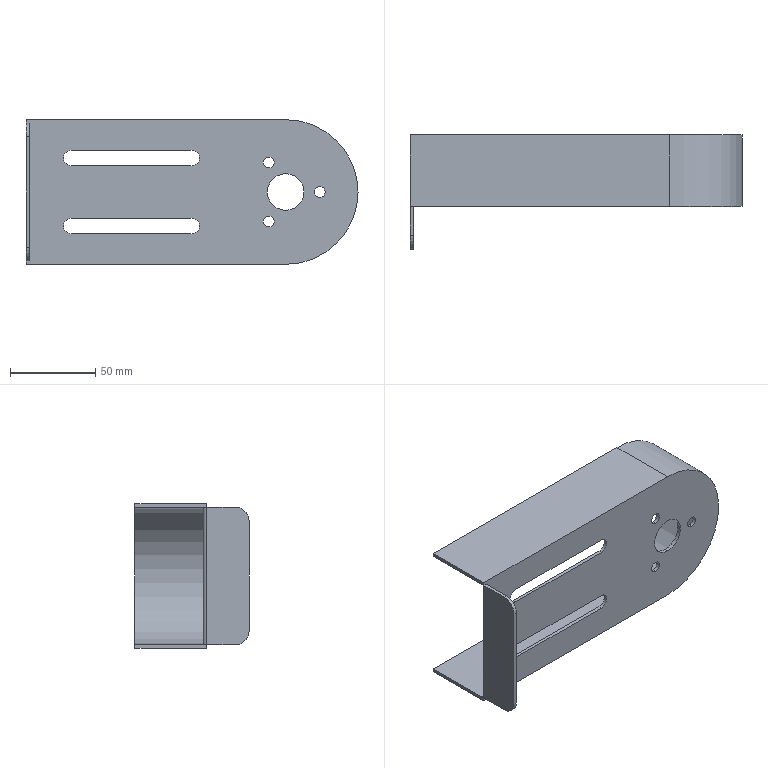Part | STEP file | 1.6米轴盖 | 1 solid | 35 faces | box 195 x 67 x 85 mm | volume 66626 mm3 | plane 18 | cylinder 17 | commonest cylinder face diameters 6.4 x6 9 x4 16 x2 21.5 x2 4 x1 81 x1
STEP:
#1=CARTESIAN_POINT('',(142.5,2.,-21.979));
#2=VERTEX_POINT('',#1);
#3=CARTESIAN_POINT('',(142.5,2.,-28.379));
#4=VERTEX_POINT('',#3);
#5=CARTESIAN_POINT('',(142.5,2.,-25.179));
#6=DIRECTION('',(0.,-1.,0.));
#7=DIRECTION('',(0.,0.,-1.));
#8=AXIS2_PLACEMENT_3D('',#5,#6,#7);
#9=CIRCLE('',#8,3.2);
#10=EDGE_CURVE('',#2,#4,#9,.T.);
#11=ORIENTED_EDGE('',*,*,#10,.F.);
#12=CARTESIAN_POINT('',(142.5,0.,-21.979));
#13=VERTEX_POINT('',#12);
#14=CARTESIAN_POINT('',(142.5,2.,-21.979));
#15=DIRECTION('',(0.,-1.,0.));
#16=VECTOR('',#15,1000.);
#17=LINE('',#14,#16);
#18=EDGE_CURVE('',#2,#13,#17,.T.);
#19=ORIENTED_EDGE('',*,*,#18,.T.);
#20=CARTESIAN_POINT('',(142.5,0.,-28.379));
#21=VERTEX_POINT('',#20);
#22=CARTESIAN_POINT('',(142.5,0.,-25.179));
#23=DIRECTION('',(0.,-1.,0.));
#24=DIRECTION('',(0.,0.,-1.));
#25=AXIS2_PLACEMENT_3D('',#22,#23,#24);
#26=CIRCLE('',#25,3.2);
#27=EDGE_CURVE('',#13,#21,#26,.T.);
#28=ORIENTED_EDGE('',*,*,#27,.T.);
#29=CARTESIAN_POINT('',(142.5,2.,-28.379));
#30=DIRECTION('',(0.,-1.,0.));
#31=VECTOR('',#30,1000.);
#32=LINE('',#29,#31);
#33=EDGE_CURVE('',#4,#21,#32,.T.);
#34=ORIENTED_EDGE('',*,*,#33,.F.);
#35=EDGE_LOOP('',(#11,#19,#28,#34));
#36=FACE_OUTER_BOUND('',#35,.T.);
#37=CARTESIAN_POINT('',(142.5,2.,-25.179));
#38=DIRECTION('',(0.,-1.,0.));
#39=DIRECTION('',(0.,0.,-1.));
#40=AXIS2_PLACEMENT_3D('',#37,#38,#39);
#41=CYLINDRICAL_SURFACE('',#40,3.2);
#42=ADVANCED_FACE('',(#36),#41,.F.);
#43=CARTESIAN_POINT('',(142.5,2.,-56.621));
#44=VERTEX_POINT('',#43);
#45=CARTESIAN_POINT('',(142.5,2.,-63.021));
#46=VERTEX_POINT('',#45);
#47=CARTESIAN_POINT('',(142.5,2.,-59.821));
#48=DIRECTION('',(0.,-1.,0.));
#49=DIRECTION('',(0.,0.,-1.));
#50=AXIS2_PLACEMENT_3D('',#47,#48,#49);
#51=CIRCLE('',#50,3.2);
#52=EDGE_CURVE('',#44,#46,#51,.T.);
#53=ORIENTED_EDGE('',*,*,#52,.F.);
#54=CARTESIAN_POINT('',(142.5,0.,-56.621));
#55=VERTEX_POINT('',#54);
#56=CARTESIAN_POINT('',(142.5,2.,-56.621));
#57=DIRECTION('',(0.,-1.,0.));
#58=VECTOR('',#57,1000.);
#59=LINE('',#56,#58);
#60=EDGE_CURVE('',#44,#55,#59,.T.);
#61=ORIENTED_EDGE('',*,*,#60,.T.);
#62=CARTESIAN_POINT('',(142.5,0.,-63.021));
#63=VERTEX_POINT('',#62);
#64=CARTESIAN_POINT('',(142.5,0.,-59.821));
#65=DIRECTION('',(0.,-1.,0.));
#66=DIRECTION('',(0.,0.,-1.));
#67=AXIS2_PLACEMENT_3D('',#64,#65,#66);
#68=CIRCLE('',#67,3.2);
#69=EDGE_CURVE('',#55,#63,#68,.T.);
#70=ORIENTED_EDGE('',*,*,#69,.T.);
#71=CARTESIAN_POINT('',(142.5,2.,-63.021));
#72=DIRECTION('',(0.,-1.,0.));
#73=VECTOR('',#72,1000.);
#74=LINE('',#71,#73);
#75=EDGE_CURVE('',#46,#63,#74,.T.);
#76=ORIENTED_EDGE('',*,*,#75,.F.);
#77=EDGE_LOOP('',(#53,#61,#70,#76));
#78=FACE_OUTER_BOUND('',#77,.T.);
#79=CARTESIAN_POINT('',(142.5,2.,-59.821));
#80=DIRECTION('',(0.,-1.,0.));
#81=DIRECTION('',(0.,0.,-1.));
#82=AXIS2_PLACEMENT_3D('',#79,#80,#81);
#83=CYLINDRICAL_SURFACE('',#82,3.2);
#84=ADVANCED_FACE('',(#78),#83,.F.);
#85=CARTESIAN_POINT('',(172.5,2.,-39.3));
#86=VERTEX_POINT('',#85);
#87=CARTESIAN_POINT('',(172.5,2.,-45.7));
#88=VERTEX_POINT('',#87);
#89=CARTESIAN_POINT('',(172.5,2.,-42.5));
#90=DIRECTION('',(0.,-1.,0.));
#91=DIRECTION('',(0.,0.,-1.));
#92=AXIS2_PLACEMENT_3D('',#89,#90,#91);
#93=CIRCLE('',#92,3.2);
#94=EDGE_CURVE('',#86,#88,#93,.T.);
#95=ORIENTED_EDGE('',*,*,#94,.F.);
#96=CARTESIAN_POINT('',(172.5,0.,-39.3));
#97=VERTEX_POINT('',#96);
#98=CARTESIAN_POINT('',(172.5,2.,-39.3));
#99=DIRECTION('',(0.,-1.,0.));
#100=VECTOR('',#99,1000.);
#101=LINE('',#98,#100);
#102=EDGE_CURVE('',#86,#97,#101,.T.);
#103=ORIENTED_EDGE('',*,*,#102,.T.);
#104=CARTESIAN_POINT('',(172.5,0.,-45.7));
#105=VERTEX_POINT('',#104);
#106=CARTESIAN_POINT('',(172.5,0.,-42.5));
#107=DIRECTION('',(0.,-1.,0.));
#108=DIRECTION('',(0.,0.,-1.));
#109=AXIS2_PLACEMENT_3D('',#106,#107,#108);
#110=CIRCLE('',#109,3.2);
#111=EDGE_CURVE('',#97,#105,#110,.T.);
#112=ORIENTED_EDGE('',*,*,#111,.T.);
#113=CARTESIAN_POINT('',(172.5,2.,-45.7));
#114=DIRECTION('',(0.,-1.,0.));
#115=VECTOR('',#114,1000.);
#116=LINE('',#113,#115);
#117=EDGE_CURVE('',#88,#105,#116,.T.);
#118=ORIENTED_EDGE('',*,*,#117,.F.);
#119=EDGE_LOOP('',(#95,#103,#112,#118));
#120=FACE_OUTER_BOUND('',#119,.T.);
#121=CARTESIAN_POINT('',(172.5,2.,-42.5));
#122=DIRECTION('',(0.,-1.,0.));
#123=DIRECTION('',(0.,0.,-1.));
#124=AXIS2_PLACEMENT_3D('',#121,#122,#123);
#125=CYLINDRICAL_SURFACE('',#124,3.2);
#126=ADVANCED_FACE('',(#120),#125,.F.);
#127=CARTESIAN_POINT('',(152.5,2.,-31.75));
#128=VERTEX_POINT('',#127);
#129=CARTESIAN_POINT('',(152.5,2.,-53.25));
#130=VERTEX_POINT('',#129);
#131=CARTESIAN_POINT('',(152.5,2.,-42.5));
#132=DIRECTION('',(0.,-1.,0.));
#133=DIRECTION('',(0.,0.,-1.));
#134=AXIS2_PLACEMENT_3D('',#131,#132,#133);
#135=CIRCLE('',#134,10.75);
#136=EDGE_CURVE('',#128,#130,#135,.T.);
#137=ORIENTED_EDGE('',*,*,#136,.F.);
#138=CARTESIAN_POINT('',(152.5,0.,-31.75));
#139=VERTEX_POINT('',#138);
#140=CARTESIAN_POINT('',(152.5,2.,-31.75));
#141=DIRECTION('',(0.,-1.,0.));
#142=VECTOR('',#141,1000.);
#143=LINE('',#140,#142);
#144=EDGE_CURVE('',#128,#139,#143,.T.);
#145=ORIENTED_EDGE('',*,*,#144,.T.);
#146=CARTESIAN_POINT('',(152.5,0.,-53.25));
#147=VERTEX_POINT('',#146);
#148=CARTESIAN_POINT('',(152.5,0.,-42.5));
#149=DIRECTION('',(0.,-1.,0.));
#150=DIRECTION('',(0.,0.,-1.));
#151=AXIS2_PLACEMENT_3D('',#148,#149,#150);
#152=CIRCLE('',#151,10.75);
#153=EDGE_CURVE('',#139,#147,#152,.T.);
#154=ORIENTED_EDGE('',*,*,#153,.T.);
#155=CARTESIAN_POINT('',(152.5,2.,-53.25));
#156=DIRECTION('',(0.,-1.,0.));
#157=VECTOR('',#156,1000.);
#158=LINE('',#155,#157);
#159=EDGE_CURVE('',#130,#147,#158,.T.);
#160=ORIENTED_EDGE('',*,*,#159,.F.);
#161=EDGE_LOOP('',(#137,#145,#154,#160));
#162=FACE_OUTER_BOUND('',#161,.T.);
#163=CARTESIAN_POINT('',(152.5,2.,-42.5));
#164=DIRECTION('',(0.,-1.,0.));
#165=DIRECTION('',(0.,0.,-1.));
#166=AXIS2_PLACEMENT_3D('',#163,#164,#165);
#167=CYLINDRICAL_SURFACE('',#166,10.75);
#168=ADVANCED_FACE('',(#162),#167,.F.);
#169=CARTESIAN_POINT('',(0.,0.,-2.));
#170=VERTEX_POINT('',#169);
#171=CARTESIAN_POINT('',(0.,42.,-2.));
#172=VERTEX_POINT('',#171);
#173=CARTESIAN_POINT('',(0.,2.,-2.));
#174=DIRECTION('',(0.,1.,0.));
#175=VECTOR('',#174,1000.);
#176=LINE('',#173,#175);
#177=EDGE_CURVE('',#170,#172,#176,.T.);
#178=ORIENTED_EDGE('',*,*,#177,.F.);
#179=CARTESIAN_POINT('',(0.,0.,0.));
#180=VERTEX_POINT('',#179);
#181=CARTESIAN_POINT('',(0.,0.,0.));
#182=DIRECTION('',(0.,0.,1.));
#183=VECTOR('',#182,1000.);
#184=LINE('',#181,#183);
#185=EDGE_CURVE('',#170,#180,#184,.T.);
#186=ORIENTED_EDGE('',*,*,#185,.T.);
#187=CARTESIAN_POINT('',(0.,42.,0.));
#188=VERTEX_POINT('',#187);
#189=CARTESIAN_POINT('',(0.,42.,0.));
#190=DIRECTION('',(0.,-1.,0.));
#191=VECTOR('',#190,1000.);
#192=LINE('',#189,#191);
#193=EDGE_CURVE('',#188,#180,#192,.T.);
#194=ORIENTED_EDGE('',*,*,#193,.F.);
#195=CARTESIAN_POINT('',(0.,42.,0.));
#196=DIRECTION('',(0.,0.,1.));
#197=VECTOR('',#196,1000.);
#198=LINE('',#195,#197);
#199=EDGE_CURVE('',#172,#188,#198,.T.);
#200=ORIENTED_EDGE('',*,*,#199,.F.);
#201=EDGE_LOOP('',(#178,#186,#194,#200));
#202=FACE_OUTER_BOUND('',#201,.T.);
#203=CARTESIAN_POINT('',(0.,42.,0.));
#204=DIRECTION('',(1.,0.,0.));
#205=DIRECTION('',(0.,0.,-1.));
#206=AXIS2_PLACEMENT_3D('',#203,#204,#205);
#207=PLANE('',#206);
#208=ADVANCED_FACE('',(#202),#207,.F.);
#209=CARTESIAN_POINT('',(0.,-17.,-2.));
#210=VERTEX_POINT('',#209);
#211=CARTESIAN_POINT('',(0.,2.,-2.));
#212=DIRECTION('',(0.,1.,0.));
#213=VECTOR('',#212,1000.);
#214=LINE('',#211,#213);
#215=EDGE_CURVE('',#210,#170,#214,.T.);
#216=ORIENTED_EDGE('',*,*,#215,.T.);
#217=CARTESIAN_POINT('',(0.,0.,-83.));
#218=VERTEX_POINT('',#217);
#219=CARTESIAN_POINT('',(0.,0.,-83.));
#220=DIRECTION('',(0.,0.,-1.));
#221=VECTOR('',#220,1000.);
#222=LINE('',#219,#221);
#223=EDGE_CURVE('',#170,#218,#222,.T.);
#224=ORIENTED_EDGE('',*,*,#223,.T.);
#225=CARTESIAN_POINT('',(0.,-17.,-83.));
#226=VERTEX_POINT('',#225);
#227=CARTESIAN_POINT('',(0.,2.,-83.));
#228=DIRECTION('',(0.,-1.,0.));
#229=VECTOR('',#228,1000.);
#230=LINE('',#227,#229);
#231=EDGE_CURVE('',#218,#226,#230,.T.);
#232=ORIENTED_EDGE('',*,*,#231,.T.);
#233=CARTESIAN_POINT('',(0.,-25.,-75.));
#234=VERTEX_POINT('',#233);
#235=CARTESIAN_POINT('',(0.,-17.,-75.));
#236=DIRECTION('',(-1.,0.,0.));
#237=DIRECTION('',(0.,0.,-1.));
#238=AXIS2_PLACEMENT_3D('',#235,#236,#237);
#239=CIRCLE('',#238,8.);
#240=EDGE_CURVE('',#226,#234,#239,.T.);
#241=ORIENTED_EDGE('',*,*,#240,.T.);
#242=CARTESIAN_POINT('',(0.,-25.,-10.));
#243=VERTEX_POINT('',#242);
#244=CARTESIAN_POINT('',(0.,-25.,-83.));
#245=DIRECTION('',(0.,0.,1.));
#246=VECTOR('',#245,1000.);
#247=LINE('',#244,#246);
#248=EDGE_CURVE('',#234,#243,#247,.T.);
#249=ORIENTED_EDGE('',*,*,#248,.T.);
#250=CARTESIAN_POINT('',(0.,-17.,-10.));
#251=DIRECTION('',(-1.,0.,0.));
#252=DIRECTION('',(0.,0.,-1.));
#253=AXIS2_PLACEMENT_3D('',#250,#251,#252);
#254=CIRCLE('',#253,8.);
#255=EDGE_CURVE('',#243,#210,#254,.T.);
#256=ORIENTED_EDGE('',*,*,#255,.T.);
#257=EDGE_LOOP('',(#216,#224,#232,#241,#249,#256));
#258=FACE_OUTER_BOUND('',#257,.T.);
#259=CARTESIAN_POINT('',(0.,42.,0.));
#260=DIRECTION('',(1.,0.,0.));
#261=DIRECTION('',(0.,0.,-1.));
#262=AXIS2_PLACEMENT_3D('',#259,#260,#261);
#263=PLANE('',#262);
#264=ADVANCED_FACE('',(#258),#263,.F.);
#265=CARTESIAN_POINT('',(0.,0.,-85.));
#266=VERTEX_POINT('',#265);
#267=CARTESIAN_POINT('',(0.,0.,0.));
#268=DIRECTION('',(0.,0.,1.));
#269=VECTOR('',#268,1000.);
#270=LINE('',#267,#269);
#271=EDGE_CURVE('',#266,#218,#270,.T.);
#272=ORIENTED_EDGE('',*,*,#271,.T.);
#273=CARTESIAN_POINT('',(0.,42.,-83.));
#274=VERTEX_POINT('',#273);
#275=CARTESIAN_POINT('',(0.,2.,-83.));
#276=DIRECTION('',(0.,1.,0.));
#277=VECTOR('',#276,1000.);
#278=LINE('',#275,#277);
#279=EDGE_CURVE('',#218,#274,#278,.T.);
#280=ORIENTED_EDGE('',*,*,#279,.T.);
#281=CARTESIAN_POINT('',(0.,42.,-85.));
#282=VERTEX_POINT('',#281);
#283=CARTESIAN_POINT('',(0.,42.,0.));
#284=DIRECTION('',(0.,0.,1.));
#285=VECTOR('',#284,1000.);
#286=LINE('',#283,#285);
#287=EDGE_CURVE('',#282,#274,#286,.T.);
#288=ORIENTED_EDGE('',*,*,#287,.F.);
#289=CARTESIAN_POINT('',(0.,42.,-85.));
#290=DIRECTION('',(0.,-1.,0.));
#291=VECTOR('',#290,1000.);
#292=LINE('',#289,#291);
#293=EDGE_CURVE('',#282,#266,#292,.T.);
#294=ORIENTED_EDGE('',*,*,#293,.T.);
#295=EDGE_LOOP('',(#272,#280,#288,#294));
#296=FACE_OUTER_BOUND('',#295,.T.);
#297=CARTESIAN_POINT('',(0.,42.,0.));
#298=DIRECTION('',(1.,0.,0.));
#299=DIRECTION('',(0.,0.,-1.));
#300=AXIS2_PLACEMENT_3D('',#297,#298,#299);
#301=PLANE('',#300);
#302=ADVANCED_FACE('',(#296),#301,.F.);
#303=CARTESIAN_POINT('',(152.5,0.,0.));
#304=VERTEX_POINT('',#303);
#305=CARTESIAN_POINT('',(0.,0.,0.));
#306=DIRECTION('',(1.,0.,0.));
#307=VECTOR('',#306,1000.);
#308=LINE('',#305,#307);
#309=EDGE_CURVE('',#180,#304,#308,.T.);
#310=ORIENTED_EDGE('',*,*,#309,.T.);
#311=CARTESIAN_POINT('',(152.5,42.,0.));
#312=VERTEX_POINT('',#311);
#313=CARTESIAN_POINT('',(152.5,42.,0.));
#314=DIRECTION('',(0.,-1.,0.));
#315=VECTOR('',#314,1000.);
#316=LINE('',#313,#315);
#317=EDGE_CURVE('',#312,#304,#316,.T.);
#318=ORIENTED_EDGE('',*,*,#317,.F.);
#319=CARTESIAN_POINT('',(0.,42.,0.));
#320=DIRECTION('',(1.,0.,0.));
#321=VECTOR('',#320,1000.);
#322=LINE('',#319,#321);
#323=EDGE_CURVE('',#188,#312,#322,.T.);
#324=ORIENTED_EDGE('',*,*,#323,.F.);
#325=ORIENTED_EDGE('',*,*,#193,.T.);
#326=EDGE_LOOP('',(#310,#318,#324,#325));
#327=FACE_OUTER_BOUND('',#326,.T.);
#328=CARTESIAN_POINT('',(0.,42.,0.));
#329=DIRECTION('',(0.,0.,-1.));
#330=DIRECTION('',(-1.,0.,0.));
#331=AXIS2_PLACEMENT_3D('',#328,#329,#330);
#332=PLANE('',#331);
#333=ADVANCED_FACE('',(#327),#332,.F.);
#334=CARTESIAN_POINT('',(152.5,0.,-85.));
#335=VERTEX_POINT('',#334);
#336=CARTESIAN_POINT('',(152.5,0.,-42.5));
#337=DIRECTION('',(0.,1.,0.));
#338=DIRECTION('',(0.,0.,1.));
#339=AXIS2_PLACEMENT_3D('',#336,#337,#338);
#340=CIRCLE('',#339,42.5);
#341=EDGE_CURVE('',#304,#335,#340,.T.);
#342=ORIENTED_EDGE('',*,*,#341,.T.);
#343=CARTESIAN_POINT('',(152.5,42.,-85.));
#344=VERTEX_POINT('',#343);
#345=CARTESIAN_POINT('',(152.5,42.,-85.));
#346=DIRECTION('',(0.,-1.,0.));
#347=VECTOR('',#346,1000.);
#348=LINE('',#345,#347);
#349=EDGE_CURVE('',#344,#335,#348,.T.);
#350=ORIENTED_EDGE('',*,*,#349,.F.);
#351=CARTESIAN_POINT('',(152.5,42.,-42.5));
#352=DIRECTION('',(0.,1.,0.));
#353=DIRECTION('',(0.,0.,1.));
#354=AXIS2_PLACEMENT_3D('',#351,#352,#353);
#355=CIRCLE('',#354,42.5);
#356=EDGE_CURVE('',#312,#344,#355,.T.);
#357=ORIENTED_EDGE('',*,*,#356,.F.);
#358=ORIENTED_EDGE('',*,*,#317,.T.);
#359=EDGE_LOOP('',(#342,#350,#357,#358));
#360=FACE_OUTER_BOUND('',#359,.T.);
#361=CARTESIAN_POINT('',(152.5,42.,-42.5));
#362=DIRECTION('',(0.,-1.,0.));
#363=DIRECTION('',(0.,0.,-1.));
#364=AXIS2_PLACEMENT_3D('',#361,#362,#363);
#365=CYLINDRICAL_SURFACE('',#364,42.5);
#366=ADVANCED_FACE('',(#360),#365,.T.);
#367=CARTESIAN_POINT('',(0.,0.,-85.));
#368=DIRECTION('',(-1.,0.,0.));
#369=VECTOR('',#368,1000.);
#370=LINE('',#367,#369);
#371=EDGE_CURVE('',#335,#266,#370,.T.);
#372=ORIENTED_EDGE('',*,*,#371,.T.);
#373=ORIENTED_EDGE('',*,*,#293,.F.);
#374=CARTESIAN_POINT('',(0.,42.,-85.));
#375=DIRECTION('',(-1.,0.,0.));
#376=VECTOR('',#375,1000.);
#377=LINE('',#374,#376);
#378=EDGE_CURVE('',#344,#282,#377,.T.);
#379=ORIENTED_EDGE('',*,*,#378,.F.);
#380=ORIENTED_EDGE('',*,*,#349,.T.);
#381=EDGE_LOOP('',(#372,#373,#379,#380));
#382=FACE_OUTER_BOUND('',#381,.T.);
#383=CARTESIAN_POINT('',(0.,42.,-85.));
#384=DIRECTION('',(0.,0.,1.));
#385=DIRECTION('',(1.,0.,0.));
#386=AXIS2_PLACEMENT_3D('',#383,#384,#385);
#387=PLANE('',#386);
#388=ADVANCED_FACE('',(#382),#387,.F.);
#389=CARTESIAN_POINT('',(152.5,42.,-2.));
#390=VERTEX_POINT('',#389);
#391=CARTESIAN_POINT('',(0.,42.,-2.));
#392=DIRECTION('',(1.,0.,0.));
#393=VECTOR('',#392,1000.);
#394=LINE('',#391,#393);
#395=EDGE_CURVE('',#172,#390,#394,.T.);
#396=ORIENTED_EDGE('',*,*,#395,.F.);
#397=ORIENTED_EDGE('',*,*,#199,.T.);
#398=ORIENTED_EDGE('',*,*,#323,.T.);
#399=ORIENTED_EDGE('',*,*,#356,.T.);
#400=ORIENTED_EDGE('',*,*,#378,.T.);
#401=ORIENTED_EDGE('',*,*,#287,.T.);
#402=CARTESIAN_POINT('',(152.5,42.,-83.));
#403=VERTEX_POINT('',#402);
#404=CARTESIAN_POINT('',(0.,42.,-83.));
#405=DIRECTION('',(-1.,0.,0.));
#406=VECTOR('',#405,1000.);
#407=LINE('',#404,#406);
#408=EDGE_CURVE('',#403,#274,#407,.T.);
#409=ORIENTED_EDGE('',*,*,#408,.F.);
#410=CARTESIAN_POINT('',(152.5,42.,-42.5));
#411=DIRECTION('',(0.,1.,0.));
#412=DIRECTION('',(0.,0.,1.));
#413=AXIS2_PLACEMENT_3D('',#410,#411,#412);
#414=CIRCLE('',#413,40.5);
#415=EDGE_CURVE('',#390,#403,#414,.T.);
#416=ORIENTED_EDGE('',*,*,#415,.F.);
#417=EDGE_LOOP('',(#396,#397,#398,#399,#400,#401,#409,#416));
#418=FACE_OUTER_BOUND('',#417,.T.);
#419=CARTESIAN_POINT('',(152.5,42.,-42.5));
#420=DIRECTION('',(0.,1.,0.));
#421=DIRECTION('',(0.,0.,1.));
#422=AXIS2_PLACEMENT_3D('',#419,#420,#421);
#423=PLANE('',#422);
#424=ADVANCED_FACE('',(#418),#423,.T.);
#425=CARTESIAN_POINT('',(26.5,0.,-67.));
#426=VERTEX_POINT('',#425);
#427=CARTESIAN_POINT('',(97.5,0.,-67.));
#428=VERTEX_POINT('',#427);
#429=CARTESIAN_POINT('',(26.5,0.,-67.));
#430=DIRECTION('',(1.,0.,0.));
#431=VECTOR('',#430,1000.);
#432=LINE('',#429,#431);
#433=EDGE_CURVE('',#426,#428,#432,.T.);
#434=ORIENTED_EDGE('',*,*,#433,.F.);
#435=CARTESIAN_POINT('',(26.5,0.,-58.));
#436=VERTEX_POINT('',#435);
#437=CARTESIAN_POINT('',(26.5,0.,-62.5));
#438=DIRECTION('',(0.,-1.,0.));
#439=DIRECTION('',(0.,0.,1.));
#440=AXIS2_PLACEMENT_3D('',#437,#438,#439);
#441=CIRCLE('',#440,4.5);
#442=EDGE_CURVE('',#436,#426,#441,.T.);
#443=ORIENTED_EDGE('',*,*,#442,.F.);
#444=CARTESIAN_POINT('',(97.5,0.,-58.));
#445=VERTEX_POINT('',#444);
#446=CARTESIAN_POINT('',(26.5,0.,-58.));
#447=DIRECTION('',(-1.,0.,0.));
#448=VECTOR('',#447,1000.);
#449=LINE('',#446,#448);
#450=EDGE_CURVE('',#445,#436,#449,.T.);
#451=ORIENTED_EDGE('',*,*,#450,.F.);
#452=CARTESIAN_POINT('',(97.5,0.,-62.5));
#453=DIRECTION('',(0.,-1.,0.));
#454=DIRECTION('',(0.,0.,1.));
#455=AXIS2_PLACEMENT_3D('',#452,#453,#454);
#456=CIRCLE('',#455,4.5);
#457=EDGE_CURVE('',#428,#445,#456,.T.);
#458=ORIENTED_EDGE('',*,*,#457,.F.);
#459=EDGE_LOOP('',(#434,#443,#451,#458));
#460=FACE_BOUND('',#459,.T.);
#461=CARTESIAN_POINT('',(26.5,0.,-27.));
#462=VERTEX_POINT('',#461);
#463=CARTESIAN_POINT('',(97.5,0.,-27.));
#464=VERTEX_POINT('',#463);
#465=CARTESIAN_POINT('',(26.5,0.,-27.));
#466=DIRECTION('',(1.,0.,0.));
#467=VECTOR('',#466,1000.);
#468=LINE('',#465,#467);
#469=EDGE_CURVE('',#462,#464,#468,.T.);
#470=ORIENTED_EDGE('',*,*,#469,.F.);
#471=CARTESIAN_POINT('',(26.5,0.,-18.));
#472=VERTEX_POINT('',#471);
#473=CARTESIAN_POINT('',(26.5,0.,-22.5));
#474=DIRECTION('',(0.,-1.,0.));
#475=DIRECTION('',(0.,0.,-1.));
#476=AXIS2_PLACEMENT_3D('',#473,#474,#475);
#477=CIRCLE('',#476,4.5);
#478=EDGE_CURVE('',#472,#462,#477,.T.);
#479=ORIENTED_EDGE('',*,*,#478,.F.);
#480=CARTESIAN_POINT('',(97.5,0.,-18.));
#481=VERTEX_POINT('',#480);
#482=CARTESIAN_POINT('',(26.5,0.,-18.));
#483=DIRECTION('',(-1.,0.,0.));
#484=VECTOR('',#483,1000.);
#485=LINE('',#482,#484);
#486=EDGE_CURVE('',#481,#472,#485,.T.);
#487=ORIENTED_EDGE('',*,*,#486,.F.);
#488=CARTESIAN_POINT('',(97.5,0.,-22.5));
#489=DIRECTION('',(0.,-1.,0.));
#490=DIRECTION('',(0.,0.,-1.));
#491=AXIS2_PLACEMENT_3D('',#488,#489,#490);
#492=CIRCLE('',#491,4.5);
#493=EDGE_CURVE('',#464,#481,#492,.T.);
#494=ORIENTED_EDGE('',*,*,#493,.F.);
#495=EDGE_LOOP('',(#470,#479,#487,#494));
#496=FACE_BOUND('',#495,.T.);
#497=CARTESIAN_POINT('',(142.5,0.,-25.179));
#498=DIRECTION('',(0.,-1.,0.));
#499=DIRECTION('',(0.,0.,-1.));
#500=AXIS2_PLACEMENT_3D('',#497,#498,#499);
#501=CIRCLE('',#500,3.2);
#502=EDGE_CURVE('',#21,#13,#501,.T.);
#503=ORIENTED_EDGE('',*,*,#502,.F.);
#504=ORIENTED_EDGE('',*,*,#27,.F.);
#505=EDGE_LOOP('',(#503,#504));
#506=FACE_BOUND('',#505,.T.);
#507=CARTESIAN_POINT('',(142.5,0.,-59.821));
#508=DIRECTION('',(0.,-1.,0.));
#509=DIRECTION('',(0.,0.,-1.));
#510=AXIS2_PLACEMENT_3D('',#507,#508,#509);
#511=CIRCLE('',#510,3.2);
#512=EDGE_CURVE('',#63,#55,#511,.T.);
#513=ORIENTED_EDGE('',*,*,#512,.F.);
#514=ORIENTED_EDGE('',*,*,#69,.F.);
#515=EDGE_LOOP('',(#513,#514));
#516=FACE_BOUND('',#515,.T.);
#517=CARTESIAN_POINT('',(172.5,0.,-42.5));
#518=DIRECTION('',(0.,-1.,0.));
#519=DIRECTION('',(0.,0.,-1.));
#520=AXIS2_PLACEMENT_3D('',#517,#518,#519);
#521=CIRCLE('',#520,3.2);
#522=EDGE_CURVE('',#105,#97,#521,.T.);
#523=ORIENTED_EDGE('',*,*,#522,.F.);
#524=ORIENTED_EDGE('',*,*,#111,.F.);
#525=EDGE_LOOP('',(#523,#524));
#526=FACE_BOUND('',#525,.T.);
#527=CARTESIAN_POINT('',(152.5,0.,-42.5));
#528=DIRECTION('',(0.,-1.,0.));
#529=DIRECTION('',(0.,0.,-1.));
#530=AXIS2_PLACEMENT_3D('',#527,#528,#529);
#531=CIRCLE('',#530,10.75);
#532=EDGE_CURVE('',#147,#139,#531,.T.);
#533=ORIENTED_EDGE('',*,*,#532,.F.);
#534=ORIENTED_EDGE('',*,*,#153,.F.);
#535=EDGE_LOOP('',(#533,#534));
#536=FACE_BOUND('',#535,.T.);
#537=CARTESIAN_POINT('',(2.,0.,-83.));
#538=VERTEX_POINT('',#537);
#539=CARTESIAN_POINT('',(2.,0.,-2.));
#540=VERTEX_POINT('',#539);
#541=CARTESIAN_POINT('',(2.,0.,-42.5));
#542=DIRECTION('',(0.,0.,1.));
#543=VECTOR('',#542,1000.);
#544=LINE('',#541,#543);
#545=EDGE_CURVE('',#538,#540,#544,.T.);
#546=ORIENTED_EDGE('',*,*,#545,.F.);
#547=CARTESIAN_POINT('',(152.5,0.,-83.));
#548=DIRECTION('',(-1.,0.,0.));
#549=VECTOR('',#548,1000.);
#550=LINE('',#547,#549);
#551=EDGE_CURVE('',#538,#218,#550,.T.);
#552=ORIENTED_EDGE('',*,*,#551,.T.);
#553=ORIENTED_EDGE('',*,*,#271,.F.);
#554=ORIENTED_EDGE('',*,*,#371,.F.);
#555=ORIENTED_EDGE('',*,*,#341,.F.);
#556=ORIENTED_EDGE('',*,*,#309,.F.);
#557=ORIENTED_EDGE('',*,*,#185,.F.);
#558=CARTESIAN_POINT('',(152.5,0.,-2.));
#559=DIRECTION('',(1.,0.,0.));
#560=VECTOR('',#559,1000.);
#561=LINE('',#558,#560);
#562=EDGE_CURVE('',#170,#540,#561,.T.);
#563=ORIENTED_EDGE('',*,*,#562,.T.);
#564=EDGE_LOOP('',(#546,#552,#553,#554,#555,#556,#557,#563));
#565=FACE_OUTER_BOUND('',#564,.T.);
#566=CARTESIAN_POINT('',(152.5,0.,-42.5));
#567=DIRECTION('',(0.,1.,0.));
#568=DIRECTION('',(0.,0.,1.));
#569=AXIS2_PLACEMENT_3D('',#566,#567,#568);
#570=PLANE('',#569);
#571=ADVANCED_FACE('',(#460,#496,#506,#516,#526,#536,#565),#570,.F.);
#572=CARTESIAN_POINT('',(2.,2.,-2.));
#573=VERTEX_POINT('',#572);
#574=CARTESIAN_POINT('',(152.5,2.,-2.));
#575=VERTEX_POINT('',#574);
#576=CARTESIAN_POINT('',(0.,2.,-2.));
#577=DIRECTION('',(1.,0.,0.));
#578=VECTOR('',#577,1000.);
#579=LINE('',#576,#578);
#580=EDGE_CURVE('',#573,#575,#579,.T.);
#581=ORIENTED_EDGE('',*,*,#580,.F.);
#582=CARTESIAN_POINT('',(2.,0.,-2.));
#583=DIRECTION('',(0.,0.,1.));
#584=DIRECTION('',(-1.,0.,0.));
#585=AXIS2_PLACEMENT_3D('',#582,#583,#584);
#586=CIRCLE('',#585,2.);
#587=EDGE_CURVE('',#573,#170,#586,.T.);
#588=ORIENTED_EDGE('',*,*,#587,.T.);
#589=ORIENTED_EDGE('',*,*,#177,.T.);
#590=ORIENTED_EDGE('',*,*,#395,.T.);
#591=CARTESIAN_POINT('',(152.5,42.,-2.));
#592=DIRECTION('',(0.,-1.,0.));
#593=VECTOR('',#592,1000.);
#594=LINE('',#591,#593);
#595=EDGE_CURVE('',#390,#575,#594,.T.);
#596=ORIENTED_EDGE('',*,*,#595,.T.);
#597=EDGE_LOOP('',(#581,#588,#589,#590,#596));
#598=FACE_OUTER_BOUND('',#597,.T.);
#599=CARTESIAN_POINT('',(0.,42.,-2.));
#600=DIRECTION('',(0.,0.,-1.));
#601=DIRECTION('',(-1.,0.,0.));
#602=AXIS2_PLACEMENT_3D('',#599,#600,#601);
#603=PLANE('',#602);
#604=ADVANCED_FACE('',(#598),#603,.T.);
#605=CARTESIAN_POINT('',(152.5,2.,-83.));
#606=VERTEX_POINT('',#605);
#607=CARTESIAN_POINT('',(152.5,2.,-42.5));
#608=DIRECTION('',(0.,1.,0.));
#609=DIRECTION('',(0.,0.,1.));
#610=AXIS2_PLACEMENT_3D('',#607,#608,#609);
#611=CIRCLE('',#610,40.5);
#612=EDGE_CURVE('',#575,#606,#611,.T.);
#613=ORIENTED_EDGE('',*,*,#612,.F.);
#614=ORIENTED_EDGE('',*,*,#595,.F.);
#615=ORIENTED_EDGE('',*,*,#415,.T.);
#616=CARTESIAN_POINT('',(152.5,42.,-83.));
#617=DIRECTION('',(0.,-1.,0.));
#618=VECTOR('',#617,1000.);
#619=LINE('',#616,#618);
#620=EDGE_CURVE('',#403,#606,#619,.T.);
#621=ORIENTED_EDGE('',*,*,#620,.T.);
#622=EDGE_LOOP('',(#613,#614,#615,#621));
#623=FACE_OUTER_BOUND('',#622,.T.);
#624=CARTESIAN_POINT('',(152.5,42.,-42.5));
#625=DIRECTION('',(0.,-1.,0.));
#626=DIRECTION('',(0.,0.,-1.));
#627=AXIS2_PLACEMENT_3D('',#624,#625,#626);
#628=CYLINDRICAL_SURFACE('',#627,40.5);
#629=ADVANCED_FACE('',(#623),#628,.F.);
#630=CARTESIAN_POINT('',(2.,2.,-83.));
#631=VERTEX_POINT('',#630);
#632=CARTESIAN_POINT('',(0.,2.,-83.));
#633=DIRECTION('',(-1.,0.,0.));
#634=VECTOR('',#633,1000.);
#635=LINE('',#632,#634);
#636=EDGE_CURVE('',#606,#631,#635,.T.);
#637=ORIENTED_EDGE('',*,*,#636,.F.);
#638=ORIENTED_EDGE('',*,*,#620,.F.);
#639=ORIENTED_EDGE('',*,*,#408,.T.);
#640=ORIENTED_EDGE('',*,*,#279,.F.);
#641=CARTESIAN_POINT('',(2.,0.,-83.));
#642=DIRECTION('',(0.,0.,-1.));
#643=DIRECTION('',(1.,0.,0.));
#644=AXIS2_PLACEMENT_3D('',#641,#642,#643);
#645=CIRCLE('',#644,2.);
#646=EDGE_CURVE('',#218,#631,#645,.T.);
#647=ORIENTED_EDGE('',*,*,#646,.T.);
#648=EDGE_LOOP('',(#637,#638,#639,#640,#647));
#649=FACE_OUTER_BOUND('',#648,.T.);
#650=CARTESIAN_POINT('',(0.,42.,-83.));
#651=DIRECTION('',(0.,0.,1.));
#652=DIRECTION('',(1.,0.,0.));
#653=AXIS2_PLACEMENT_3D('',#650,#651,#652);
#654=PLANE('',#653);
#655=ADVANCED_FACE('',(#649),#654,.T.);
#656=CARTESIAN_POINT('',(26.5,2.,-58.));
#657=VERTEX_POINT('',#656);
#658=CARTESIAN_POINT('',(26.5,2.,-67.));
#659=VERTEX_POINT('',#658);
#660=CARTESIAN_POINT('',(26.5,2.,-62.5));
#661=DIRECTION('',(0.,-1.,0.));
#662=DIRECTION('',(0.,0.,1.));
#663=AXIS2_PLACEMENT_3D('',#660,#661,#662);
#664=CIRCLE('',#663,4.5);
#665=EDGE_CURVE('',#657,#659,#664,.T.);
#666=ORIENTED_EDGE('',*,*,#665,.T.);
#667=CARTESIAN_POINT('',(97.5,2.,-67.));
#668=VERTEX_POINT('',#667);
#669=CARTESIAN_POINT('',(26.5,2.,-67.));
#670=DIRECTION('',(1.,0.,0.));
#671=VECTOR('',#670,1000.);
#672=LINE('',#669,#671);
#673=EDGE_CURVE('',#659,#668,#672,.T.);
#674=ORIENTED_EDGE('',*,*,#673,.T.);
#675=CARTESIAN_POINT('',(97.5,2.,-58.));
#676=VERTEX_POINT('',#675);
#677=CARTESIAN_POINT('',(97.5,2.,-62.5));
#678=DIRECTION('',(0.,-1.,0.));
#679=DIRECTION('',(0.,0.,1.));
#680=AXIS2_PLACEMENT_3D('',#677,#678,#679);
#681=CIRCLE('',#680,4.5);
#682=EDGE_CURVE('',#668,#676,#681,.T.);
#683=ORIENTED_EDGE('',*,*,#682,.T.);
#684=CARTESIAN_POINT('',(26.5,2.,-58.));
#685=DIRECTION('',(-1.,0.,0.));
#686=VECTOR('',#685,1000.);
#687=LINE('',#684,#686);
#688=EDGE_CURVE('',#676,#657,#687,.T.);
#689=ORIENTED_EDGE('',*,*,#688,.T.);
#690=EDGE_LOOP('',(#666,#674,#683,#689));
#691=FACE_BOUND('',#690,.T.);
#692=CARTESIAN_POINT('',(26.5,2.,-18.));
#693=VERTEX_POINT('',#692);
#694=CARTESIAN_POINT('',(26.5,2.,-27.));
#695=VERTEX_POINT('',#694);
#696=CARTESIAN_POINT('',(26.5,2.,-22.5));
#697=DIRECTION('',(0.,-1.,0.));
#698=DIRECTION('',(0.,0.,-1.));
#699=AXIS2_PLACEMENT_3D('',#696,#697,#698);
#700=CIRCLE('',#699,4.5);
#701=EDGE_CURVE('',#693,#695,#700,.T.);
#702=ORIENTED_EDGE('',*,*,#701,.T.);
#703=CARTESIAN_POINT('',(97.5,2.,-27.));
#704=VERTEX_POINT('',#703);
#705=CARTESIAN_POINT('',(26.5,2.,-27.));
#706=DIRECTION('',(1.,0.,0.));
#707=VECTOR('',#706,1000.);
#708=LINE('',#705,#707);
#709=EDGE_CURVE('',#695,#704,#708,.T.);
#710=ORIENTED_EDGE('',*,*,#709,.T.);
#711=CARTESIAN_POINT('',(97.5,2.,-18.));
#712=VERTEX_POINT('',#711);
#713=CARTESIAN_POINT('',(97.5,2.,-22.5));
#714=DIRECTION('',(0.,-1.,0.));
#715=DIRECTION('',(0.,0.,-1.));
#716=AXIS2_PLACEMENT_3D('',#713,#714,#715);
#717=CIRCLE('',#716,4.5);
#718=EDGE_CURVE('',#704,#712,#717,.T.);
#719=ORIENTED_EDGE('',*,*,#718,.T.);
#720=CARTESIAN_POINT('',(26.5,2.,-18.));
#721=DIRECTION('',(-1.,0.,0.));
#722=VECTOR('',#721,1000.);
#723=LINE('',#720,#722);
#724=EDGE_CURVE('',#712,#693,#723,.T.);
#725=ORIENTED_EDGE('',*,*,#724,.T.);
#726=EDGE_LOOP('',(#702,#710,#719,#725));
#727=FACE_BOUND('',#726,.T.);
#728=CARTESIAN_POINT('',(142.5,2.,-25.179));
#729=DIRECTION('',(0.,-1.,0.));
#730=DIRECTION('',(0.,0.,-1.));
#731=AXIS2_PLACEMENT_3D('',#728,#729,#730);
#732=CIRCLE('',#731,3.2);
#733=EDGE_CURVE('',#4,#2,#732,.T.);
#734=ORIENTED_EDGE('',*,*,#733,.T.);
#735=ORIENTED_EDGE('',*,*,#10,.T.);
#736=EDGE_LOOP('',(#734,#735));
#737=FACE_BOUND('',#736,.T.);
#738=CARTESIAN_POINT('',(142.5,2.,-59.821));
#739=DIRECTION('',(0.,-1.,0.));
#740=DIRECTION('',(0.,0.,-1.));
#741=AXIS2_PLACEMENT_3D('',#738,#739,#740);
#742=CIRCLE('',#741,3.2);
#743=EDGE_CURVE('',#46,#44,#742,.T.);
#744=ORIENTED_EDGE('',*,*,#743,.T.);
#745=ORIENTED_EDGE('',*,*,#52,.T.);
#746=EDGE_LOOP('',(#744,#745));
#747=FACE_BOUND('',#746,.T.);
#748=CARTESIAN_POINT('',(172.5,2.,-42.5));
#749=DIRECTION('',(0.,-1.,0.));
#750=DIRECTION('',(0.,0.,-1.));
#751=AXIS2_PLACEMENT_3D('',#748,#749,#750);
#752=CIRCLE('',#751,3.2);
#753=EDGE_CURVE('',#88,#86,#752,.T.);
#754=ORIENTED_EDGE('',*,*,#753,.T.);
#755=ORIENTED_EDGE('',*,*,#94,.T.);
#756=EDGE_LOOP('',(#754,#755));
#757=FACE_BOUND('',#756,.T.);
#758=CARTESIAN_POINT('',(152.5,2.,-42.5));
#759=DIRECTION('',(0.,-1.,0.));
#760=DIRECTION('',(0.,0.,-1.));
#761=AXIS2_PLACEMENT_3D('',#758,#759,#760);
#762=CIRCLE('',#761,10.75);
#763=EDGE_CURVE('',#130,#128,#762,.T.);
#764=ORIENTED_EDGE('',*,*,#763,.T.);
#765=ORIENTED_EDGE('',*,*,#136,.T.);
#766=EDGE_LOOP('',(#764,#765));
#767=FACE_BOUND('',#766,.T.);
#768=ORIENTED_EDGE('',*,*,#636,.T.);
#769=CARTESIAN_POINT('',(2.,2.,-2.));
#770=DIRECTION('',(0.,0.,1.));
#771=VECTOR('',#770,1000.);
#772=LINE('',#769,#771);
#773=EDGE_CURVE('',#631,#573,#772,.T.);
#774=ORIENTED_EDGE('',*,*,#773,.T.);
#775=ORIENTED_EDGE('',*,*,#580,.T.);
#776=ORIENTED_EDGE('',*,*,#612,.T.);
#777=EDGE_LOOP('',(#768,#774,#775,#776));
#778=FACE_OUTER_BOUND('',#777,.T.);
#779=CARTESIAN_POINT('',(152.5,2.,-42.5));
#780=DIRECTION('',(0.,1.,0.));
#781=DIRECTION('',(0.,0.,1.));
#782=AXIS2_PLACEMENT_3D('',#779,#780,#781);
#783=PLANE('',#782);
#784=ADVANCED_FACE('',(#691,#727,#737,#747,#757,#767,#778),#783,.T.);
#785=CARTESIAN_POINT('',(2.,-17.,-83.));
#786=VERTEX_POINT('',#785);
#787=CARTESIAN_POINT('',(2.,2.,-83.));
#788=DIRECTION('',(0.,-1.,0.));
#789=VECTOR('',#788,1000.);
#790=LINE('',#787,#789);
#791=EDGE_CURVE('',#538,#786,#790,.T.);
#792=ORIENTED_EDGE('',*,*,#791,.T.);
#793=CARTESIAN_POINT('',(2.,-17.,-83.));
#794=DIRECTION('',(-1.,0.,0.));
#795=VECTOR('',#794,1000.);
#796=LINE('',#793,#795);
#797=EDGE_CURVE('',#786,#226,#796,.T.);
#798=ORIENTED_EDGE('',*,*,#797,.T.);
#799=ORIENTED_EDGE('',*,*,#231,.F.);
#800=ORIENTED_EDGE('',*,*,#551,.F.);
#801=EDGE_LOOP('',(#792,#798,#799,#800));
#802=FACE_OUTER_BOUND('',#801,.T.);
#803=CARTESIAN_POINT('',(2.,2.,-83.));
#804=DIRECTION('',(0.,0.,-1.));
#805=DIRECTION('',(-1.,0.,0.));
#806=AXIS2_PLACEMENT_3D('',#803,#804,#805);
#807=PLANE('',#806);
#808=ADVANCED_FACE('',(#802),#807,.T.);
#809=ORIENTED_EDGE('',*,*,#215,.F.);
#810=CARTESIAN_POINT('',(2.,-17.,-2.));
#811=VERTEX_POINT('',#810);
#812=CARTESIAN_POINT('',(2.,-17.,-2.));
#813=DIRECTION('',(1.,0.,0.));
#814=VECTOR('',#813,1000.);
#815=LINE('',#812,#814);
#816=EDGE_CURVE('',#210,#811,#815,.T.);
#817=ORIENTED_EDGE('',*,*,#816,.T.);
#818=CARTESIAN_POINT('',(2.,2.,-2.));
#819=DIRECTION('',(0.,1.,0.));
#820=VECTOR('',#819,1000.);
#821=LINE('',#818,#820);
#822=EDGE_CURVE('',#811,#540,#821,.T.);
#823=ORIENTED_EDGE('',*,*,#822,.T.);
#824=ORIENTED_EDGE('',*,*,#562,.F.);
#825=EDGE_LOOP('',(#809,#817,#823,#824));
#826=FACE_OUTER_BOUND('',#825,.T.);
#827=CARTESIAN_POINT('',(2.,2.,-2.));
#828=DIRECTION('',(0.,0.,1.));
#829=DIRECTION('',(1.,0.,0.));
#830=AXIS2_PLACEMENT_3D('',#827,#828,#829);
#831=PLANE('',#830);
#832=ADVANCED_FACE('',(#826),#831,.T.);
#833=CARTESIAN_POINT('',(2.,-25.,-75.));
#834=VERTEX_POINT('',#833);
#835=CARTESIAN_POINT('',(2.,-25.,-10.));
#836=VERTEX_POINT('',#835);
#837=CARTESIAN_POINT('',(2.,-25.,-83.));
#838=DIRECTION('',(0.,0.,1.));
#839=VECTOR('',#838,1000.);
#840=LINE('',#837,#839);
#841=EDGE_CURVE('',#834,#836,#840,.T.);
#842=ORIENTED_EDGE('',*,*,#841,.F.);
#843=CARTESIAN_POINT('',(2.,-17.,-75.));
#844=DIRECTION('',(1.,0.,0.));
#845=DIRECTION('',(0.,0.,1.));
#846=AXIS2_PLACEMENT_3D('',#843,#844,#845);
#847=CIRCLE('',#846,8.);
#848=EDGE_CURVE('',#834,#786,#847,.T.);
#849=ORIENTED_EDGE('',*,*,#848,.T.);
#850=ORIENTED_EDGE('',*,*,#791,.F.);
#851=ORIENTED_EDGE('',*,*,#545,.T.);
#852=ORIENTED_EDGE('',*,*,#822,.F.);
#853=CARTESIAN_POINT('',(2.,-17.,-10.));
#854=DIRECTION('',(1.,0.,0.));
#855=DIRECTION('',(0.,0.,1.));
#856=AXIS2_PLACEMENT_3D('',#853,#854,#855);
#857=CIRCLE('',#856,8.);
#858=EDGE_CURVE('',#811,#836,#857,.T.);
#859=ORIENTED_EDGE('',*,*,#858,.T.);
#860=EDGE_LOOP('',(#842,#849,#850,#851,#852,#859));
#861=FACE_OUTER_BOUND('',#860,.T.);
#862=CARTESIAN_POINT('',(2.,0.,0.));
#863=DIRECTION('',(-1.,0.,0.));
#864=DIRECTION('',(0.,0.,1.));
#865=AXIS2_PLACEMENT_3D('',#862,#863,#864);
#866=PLANE('',#865);
#867=ADVANCED_FACE('',(#861),#866,.F.);
#868=ORIENTED_EDGE('',*,*,#248,.F.);
#869=CARTESIAN_POINT('',(2.,-25.,-75.));
#870=DIRECTION('',(1.,0.,0.));
#871=VECTOR('',#870,1000.);
#872=LINE('',#869,#871);
#873=EDGE_CURVE('',#234,#834,#872,.T.);
#874=ORIENTED_EDGE('',*,*,#873,.T.);
#875=ORIENTED_EDGE('',*,*,#841,.T.);
#876=CARTESIAN_POINT('',(2.,-25.,-10.));
#877=DIRECTION('',(-1.,0.,0.));
#878=VECTOR('',#877,1000.);
#879=LINE('',#876,#878);
#880=EDGE_CURVE('',#836,#243,#879,.T.);
#881=ORIENTED_EDGE('',*,*,#880,.T.);
#882=EDGE_LOOP('',(#868,#874,#875,#881));
#883=FACE_OUTER_BOUND('',#882,.T.);
#884=CARTESIAN_POINT('',(2.,-25.,-83.));
#885=DIRECTION('',(0.,-1.,0.));
#886=DIRECTION('',(0.,0.,-1.));
#887=AXIS2_PLACEMENT_3D('',#884,#885,#886);
#888=PLANE('',#887);
#889=ADVANCED_FACE('',(#883),#888,.T.);
#890=ORIENTED_EDGE('',*,*,#848,.F.);
#891=ORIENTED_EDGE('',*,*,#873,.F.);
#892=ORIENTED_EDGE('',*,*,#240,.F.);
#893=ORIENTED_EDGE('',*,*,#797,.F.);
#894=EDGE_LOOP('',(#890,#891,#892,#893));
#895=FACE_OUTER_BOUND('',#894,.T.);
#896=CARTESIAN_POINT('',(2.,-17.,-75.));
#897=DIRECTION('',(-1.,0.,0.));
#898=DIRECTION('',(0.,0.,1.));
#899=AXIS2_PLACEMENT_3D('',#896,#897,#898);
#900=CYLINDRICAL_SURFACE('',#899,8.);
#901=ADVANCED_FACE('',(#895),#900,.T.);
#902=ORIENTED_EDGE('',*,*,#858,.F.);
#903=ORIENTED_EDGE('',*,*,#816,.F.);
#904=ORIENTED_EDGE('',*,*,#255,.F.);
#905=ORIENTED_EDGE('',*,*,#880,.F.);
#906=EDGE_LOOP('',(#902,#903,#904,#905));
#907=FACE_OUTER_BOUND('',#906,.T.);
#908=CARTESIAN_POINT('',(2.,-17.,-10.));
#909=DIRECTION('',(-1.,0.,0.));
#910=DIRECTION('',(0.,0.,1.));
#911=AXIS2_PLACEMENT_3D('',#908,#909,#910);
#912=CYLINDRICAL_SURFACE('',#911,8.);
#913=ADVANCED_FACE('',(#907),#912,.T.);
#914=ORIENTED_EDGE('',*,*,#646,.F.);
#915=ORIENTED_EDGE('',*,*,#223,.F.);
#916=ORIENTED_EDGE('',*,*,#587,.F.);
#917=ORIENTED_EDGE('',*,*,#773,.F.);
#918=EDGE_LOOP('',(#914,#915,#916,#917));
#919=FACE_OUTER_BOUND('',#918,.T.);
#920=CARTESIAN_POINT('',(2.,0.,-42.5));
#921=DIRECTION('',(0.,0.,-1.));
#922=DIRECTION('',(-1.,0.,0.));
#923=AXIS2_PLACEMENT_3D('',#920,#921,#922);
#924=CYLINDRICAL_SURFACE('',#923,2.);
#925=ADVANCED_FACE('',(#919),#924,.T.);
#926=ORIENTED_EDGE('',*,*,#144,.F.);
#927=ORIENTED_EDGE('',*,*,#763,.F.);
#928=ORIENTED_EDGE('',*,*,#159,.T.);
#929=ORIENTED_EDGE('',*,*,#532,.T.);
#930=EDGE_LOOP('',(#926,#927,#928,#929));
#931=FACE_OUTER_BOUND('',#930,.T.);
#932=CARTESIAN_POINT('',(152.5,2.,-42.5));
#933=DIRECTION('',(0.,-1.,0.));
#934=DIRECTION('',(0.,0.,-1.));
#935=AXIS2_PLACEMENT_3D('',#932,#933,#934);
#936=CYLINDRICAL_SURFACE('',#935,10.75);
#937=ADVANCED_FACE('',(#931),#936,.F.);
#938=ORIENTED_EDGE('',*,*,#102,.F.);
#939=ORIENTED_EDGE('',*,*,#753,.F.);
#940=ORIENTED_EDGE('',*,*,#117,.T.);
#941=ORIENTED_EDGE('',*,*,#522,.T.);
#942=EDGE_LOOP('',(#938,#939,#940,#941));
#943=FACE_OUTER_BOUND('',#942,.T.);
#944=CARTESIAN_POINT('',(172.5,2.,-42.5));
#945=DIRECTION('',(0.,-1.,0.));
#946=DIRECTION('',(0.,0.,-1.));
#947=AXIS2_PLACEMENT_3D('',#944,#945,#946);
#948=CYLINDRICAL_SURFACE('',#947,3.2);
#949=ADVANCED_FACE('',(#943),#948,.F.);
#950=ORIENTED_EDGE('',*,*,#60,.F.);
#951=ORIENTED_EDGE('',*,*,#743,.F.);
#952=ORIENTED_EDGE('',*,*,#75,.T.);
#953=ORIENTED_EDGE('',*,*,#512,.T.);
#954=EDGE_LOOP('',(#950,#951,#952,#953));
#955=FACE_OUTER_BOUND('',#954,.T.);
#956=CARTESIAN_POINT('',(142.5,2.,-59.821));
#957=DIRECTION('',(0.,-1.,0.));
#958=DIRECTION('',(0.,0.,-1.));
#959=AXIS2_PLACEMENT_3D('',#956,#957,#958);
#960=CYLINDRICAL_SURFACE('',#959,3.2);
#961=ADVANCED_FACE('',(#955),#960,.F.);
#962=ORIENTED_EDGE('',*,*,#18,.F.);
#963=ORIENTED_EDGE('',*,*,#733,.F.);
#964=ORIENTED_EDGE('',*,*,#33,.T.);
#965=ORIENTED_EDGE('',*,*,#502,.T.);
#966=EDGE_LOOP('',(#962,#963,#964,#965));
#967=FACE_OUTER_BOUND('',#966,.T.);
#968=CARTESIAN_POINT('',(142.5,2.,-25.179));
#969=DIRECTION('',(0.,-1.,0.));
#970=DIRECTION('',(0.,0.,-1.));
#971=AXIS2_PLACEMENT_3D('',#968,#969,#970);
#972=CYLINDRICAL_SURFACE('',#971,3.2);
#973=ADVANCED_FACE('',(#967),#972,.F.);
#974=ORIENTED_EDGE('',*,*,#478,.T.);
#975=CARTESIAN_POINT('',(26.5,2.,-27.));
#976=DIRECTION('',(0.,-1.,0.));
#977=VECTOR('',#976,1000.);
#978=LINE('',#975,#977);
#979=EDGE_CURVE('',#695,#462,#978,.T.);
#980=ORIENTED_EDGE('',*,*,#979,.F.);
#981=ORIENTED_EDGE('',*,*,#701,.F.);
#982=CARTESIAN_POINT('',(26.5,2.,-18.));
#983=DIRECTION('',(0.,-1.,0.));
#984=VECTOR('',#983,1000.);
#985=LINE('',#982,#984);
#986=EDGE_CURVE('',#693,#472,#985,.T.);
#987=ORIENTED_EDGE('',*,*,#986,.T.);
#988=EDGE_LOOP('',(#974,#980,#981,#987));
#989=FACE_OUTER_BOUND('',#988,.T.);
#990=CARTESIAN_POINT('',(26.5,2.,-22.5));
#991=DIRECTION('',(0.,-1.,0.));
#992=DIRECTION('',(0.,0.,-1.));
#993=AXIS2_PLACEMENT_3D('',#990,#991,#992);
#994=CYLINDRICAL_SURFACE('',#993,4.5);
#995=ADVANCED_FACE('',(#989),#994,.F.);
#996=ORIENTED_EDGE('',*,*,#486,.T.);
#997=ORIENTED_EDGE('',*,*,#986,.F.);
#998=ORIENTED_EDGE('',*,*,#724,.F.);
#999=CARTESIAN_POINT('',(97.5,2.,-18.));
#1000=DIRECTION('',(0.,-1.,0.));
#1001=VECTOR('',#1000,1000.);
#1002=LINE('',#999,#1001);
#1003=EDGE_CURVE('',#712,#481,#1002,.T.);
#1004=ORIENTED_EDGE('',*,*,#1003,.T.);
#1005=EDGE_LOOP('',(#996,#997,#998,#1004));
#1006=FACE_OUTER_BOUND('',#1005,.T.);
#1007=CARTESIAN_POINT('',(26.5,2.,-18.));
#1008=DIRECTION('',(0.,0.,1.));
#1009=DIRECTION('',(1.,0.,0.));
#1010=AXIS2_PLACEMENT_3D('',#1007,#1008,#1009);
#1011=PLANE('',#1010);
#1012=ADVANCED_FACE('',(#1006),#1011,.F.);
#1013=ORIENTED_EDGE('',*,*,#493,.T.);
#1014=ORIENTED_EDGE('',*,*,#1003,.F.);
#1015=ORIENTED_EDGE('',*,*,#718,.F.);
#1016=CARTESIAN_POINT('',(97.5,2.,-27.));
#1017=DIRECTION('',(0.,-1.,0.));
#1018=VECTOR('',#1017,1000.);
#1019=LINE('',#1016,#1018);
#1020=EDGE_CURVE('',#704,#464,#1019,.T.);
#1021=ORIENTED_EDGE('',*,*,#1020,.T.);
#1022=EDGE_LOOP('',(#1013,#1014,#1015,#1021));
#1023=FACE_OUTER_BOUND('',#1022,.T.);
#1024=CARTESIAN_POINT('',(97.5,2.,-22.5));
#1025=DIRECTION('',(0.,-1.,0.));
#1026=DIRECTION('',(0.,0.,-1.));
#1027=AXIS2_PLACEMENT_3D('',#1024,#1025,#1026);
#1028=CYLINDRICAL_SURFACE('',#1027,4.5);
#1029=ADVANCED_FACE('',(#1023),#1028,.F.);
#1030=ORIENTED_EDGE('',*,*,#469,.T.);
#1031=ORIENTED_EDGE('',*,*,#1020,.F.);
#1032=ORIENTED_EDGE('',*,*,#709,.F.);
#1033=ORIENTED_EDGE('',*,*,#979,.T.);
#1034=EDGE_LOOP('',(#1030,#1031,#1032,#1033));
#1035=FACE_OUTER_BOUND('',#1034,.T.);
#1036=CARTESIAN_POINT('',(26.5,2.,-27.));
#1037=DIRECTION('',(0.,0.,-1.));
#1038=DIRECTION('',(-1.,0.,0.));
#1039=AXIS2_PLACEMENT_3D('',#1036,#1037,#1038);
#1040=PLANE('',#1039);
#1041=ADVANCED_FACE('',(#1035),#1040,.F.);
#1042=ORIENTED_EDGE('',*,*,#442,.T.);
#1043=CARTESIAN_POINT('',(26.5,2.,-67.));
#1044=DIRECTION('',(0.,-1.,0.));
#1045=VECTOR('',#1044,1000.);
#1046=LINE('',#1043,#1045);
#1047=EDGE_CURVE('',#659,#426,#1046,.T.);
#1048=ORIENTED_EDGE('',*,*,#1047,.F.);
#1049=ORIENTED_EDGE('',*,*,#665,.F.);
#1050=CARTESIAN_POINT('',(26.5,2.,-58.));
#1051=DIRECTION('',(0.,-1.,0.));
#1052=VECTOR('',#1051,1000.);
#1053=LINE('',#1050,#1052);
#1054=EDGE_CURVE('',#657,#436,#1053,.T.);
#1055=ORIENTED_EDGE('',*,*,#1054,.T.);
#1056=EDGE_LOOP('',(#1042,#1048,#1049,#1055));
#1057=FACE_OUTER_BOUND('',#1056,.T.);
#1058=CARTESIAN_POINT('',(26.5,2.,-62.5));
#1059=DIRECTION('',(0.,-1.,0.));
#1060=DIRECTION('',(0.,0.,-1.));
#1061=AXIS2_PLACEMENT_3D('',#1058,#1059,#1060);
#1062=CYLINDRICAL_SURFACE('',#1061,4.5);
#1063=ADVANCED_FACE('',(#1057),#1062,.F.);
#1064=ORIENTED_EDGE('',*,*,#450,.T.);
#1065=ORIENTED_EDGE('',*,*,#1054,.F.);
#1066=ORIENTED_EDGE('',*,*,#688,.F.);
#1067=CARTESIAN_POINT('',(97.5,2.,-58.));
#1068=DIRECTION('',(0.,-1.,0.));
#1069=VECTOR('',#1068,1000.);
#1070=LINE('',#1067,#1069);
#1071=EDGE_CURVE('',#676,#445,#1070,.T.);
#1072=ORIENTED_EDGE('',*,*,#1071,.T.);
#1073=EDGE_LOOP('',(#1064,#1065,#1066,#1072));
#1074=FACE_OUTER_BOUND('',#1073,.T.);
#1075=CARTESIAN_POINT('',(26.5,2.,-58.));
#1076=DIRECTION('',(0.,0.,1.));
#1077=DIRECTION('',(1.,0.,0.));
#1078=AXIS2_PLACEMENT_3D('',#1075,#1076,#1077);
#1079=PLANE('',#1078);
#1080=ADVANCED_FACE('',(#1074),#1079,.F.);
#1081=ORIENTED_EDGE('',*,*,#457,.T.);
#1082=ORIENTED_EDGE('',*,*,#1071,.F.);
#1083=ORIENTED_EDGE('',*,*,#682,.F.);
#1084=CARTESIAN_POINT('',(97.5,2.,-67.));
#1085=DIRECTION('',(0.,-1.,0.));
#1086=VECTOR('',#1085,1000.);
#1087=LINE('',#1084,#1086);
#1088=EDGE_CURVE('',#668,#428,#1087,.T.);
#1089=ORIENTED_EDGE('',*,*,#1088,.T.);
#1090=EDGE_LOOP('',(#1081,#1082,#1083,#1089));
#1091=FACE_OUTER_BOUND('',#1090,.T.);
#1092=CARTESIAN_POINT('',(97.5,2.,-62.5));
#1093=DIRECTION('',(0.,-1.,0.));
#1094=DIRECTION('',(0.,0.,-1.));
#1095=AXIS2_PLACEMENT_3D('',#1092,#1093,#1094);
#1096=CYLINDRICAL_SURFACE('',#1095,4.5);
#1097=ADVANCED_FACE('',(#1091),#1096,.F.);
#1098=ORIENTED_EDGE('',*,*,#433,.T.);
#1099=ORIENTED_EDGE('',*,*,#1088,.F.);
#1100=ORIENTED_EDGE('',*,*,#673,.F.);
#1101=ORIENTED_EDGE('',*,*,#1047,.T.);
#1102=EDGE_LOOP('',(#1098,#1099,#1100,#1101));
#1103=FACE_OUTER_BOUND('',#1102,.T.);
#1104=CARTESIAN_POINT('',(26.5,2.,-67.));
#1105=DIRECTION('',(0.,0.,-1.));
#1106=DIRECTION('',(-1.,0.,0.));
#1107=AXIS2_PLACEMENT_3D('',#1104,#1105,#1106);
#1108=PLANE('',#1107);
#1109=ADVANCED_FACE('',(#1103),#1108,.F.);
#1110=CLOSED_SHELL('',(#42,#84,#126,#168,#208,#264,#302,#333,#366,#388,#424,#571,#604,#629,#655,#784,#808,#832,#867,#889,#901,#913,#925,#937,#949,#961,#973,#995,#1012,#1029,#1041,#1063,#1080,#1097,#1109));
#1111=MANIFOLD_SOLID_BREP('',#1110);
#1112=CARTESIAN_POINT('',(0.,0.,0.));
#1113=DIRECTION('',(0.,0.,1.));
#1114=DIRECTION('',(1.,0.,0.));
#1115=AXIS2_PLACEMENT_3D('',#1112,#1113,#1114);
#1116=(LENGTH_UNIT()NAMED_UNIT(*)SI_UNIT(.MILLI.,.METRE.));
#1117=UNCERTAINTY_MEASURE_WITH_UNIT(LENGTH_MEASURE(0.00001),#1116,'','');
#1118=(NAMED_UNIT(*)PLANE_ANGLE_UNIT()SI_UNIT($,.RADIAN.));
#1119=(NAMED_UNIT(*)SI_UNIT($,.STERADIAN.)SOLID_ANGLE_UNIT());
#1120=(GEOMETRIC_REPRESENTATION_CONTEXT(3)GLOBAL_UNCERTAINTY_ASSIGNED_CONTEXT((#1117))GLOBAL_UNIT_ASSIGNED_CONTEXT((#1116,#1118,#1119))REPRESENTATION_CONTEXT('',''));
#1121=ADVANCED_BREP_SHAPE_REPRESENTATION('',(#1111,#1115),#1120);